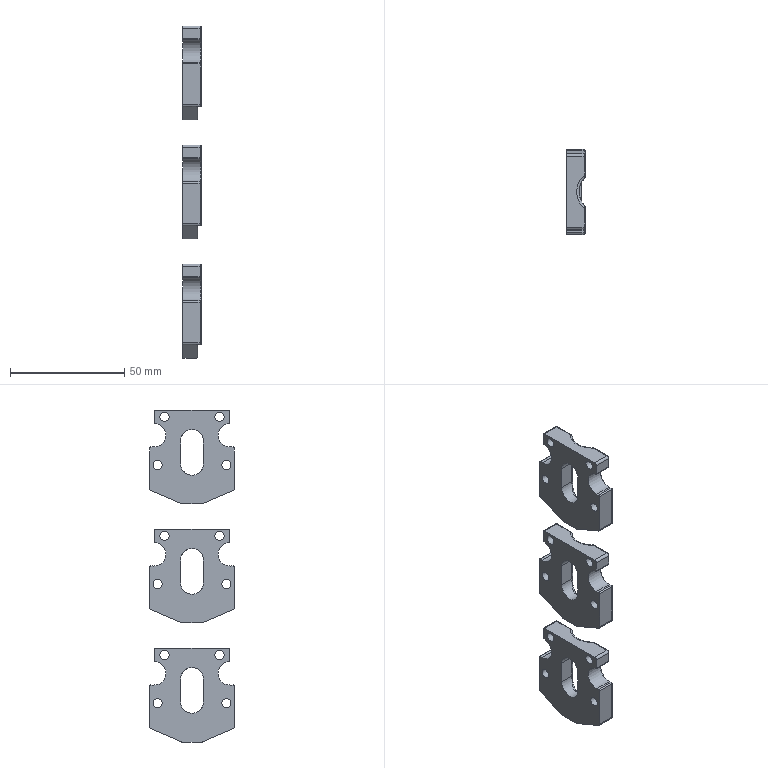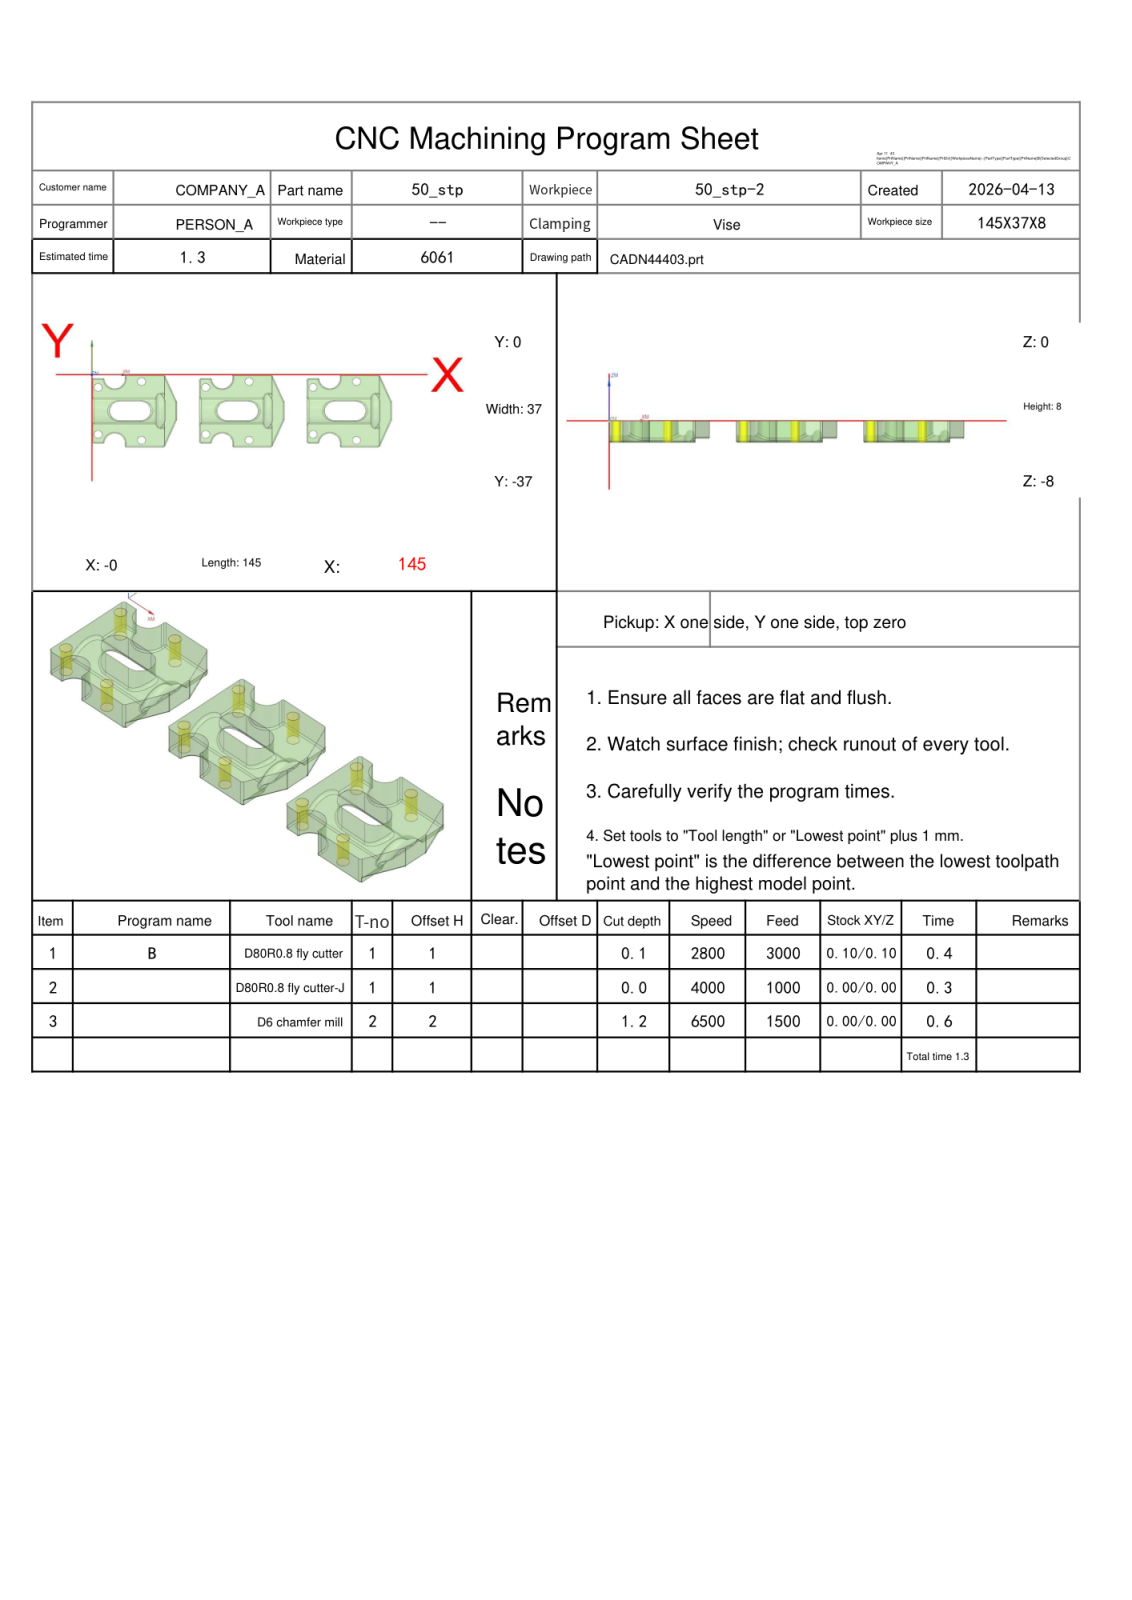NC program | NX | posted by the shop | part box 8 x 37 x 145 mm
Whole program:
%
O0001
(Machine time: 1.85 MIN)
(===Total Tool:2===)
(T1=D80R0.8 fly cutter D=80.  R=0.8  D-  H01 Z=-0.   )
(T2=D6 chamfer mill   D=6.   R=0.   D-  H02 Z=-1.2  )
G80 G90 G17 G49 G40
G91 G28 Z0
M01
N1 T01 M06
(D80R0.8 fly cutter  D=80. R=0.8 H=01 ce=0.10 di=0.10)
G00 G90 G54 X197.097 Y-18.5 M03 S2800
G43 H01 Z20.
M08
Z3.525
G01 Z1.525 F3000.
X185.097
X-40.097
X-52.097
Z3.525
G00 X197.097
Z3.05
G01 Z1.05
X185.097
X-40.097
X-52.097
Z3.05
G00 X197.097
Z2.575
G01 Z.575
X185.097
X-40.097
X-52.097
Z2.575
G00 X197.097
Z2.1
G01 Z.1
X185.097
X-40.097
X-52.097
Z2.1
G00 Z20.
G91 G28 Z0.0
M05
M09
G91 G28 Z0.0
M01
N2 T01 M06
(D80R0.8 fly cutter-J  D=80. R=0.8 H=01 ce=0.00 di=0.00)
G00 G90 G54 X196.999 Y-18.5 M03 S4000
G43 H01 Z20.
M08
Z2.
G01 Z0.0 F1000.
X184.999
X-39.999
X-51.999
Z2.
G00 Z20.
G91 G28 Z0.0
M05
M09
G91 G28 Z0.0
M01
N3 T02 M06
(D6 chamfer mill  D=6. R=0. H=02 ce=0.00 di=0.00)
G00 G90 G54 X102.773 Y-18.886 M03 S6500
G43 H02 Z20.
M08
Z.172
G01 Z-1.199 F1500.
G03 X102.973 Y-18.6 I-1.532 J1.286
G01 X103.003 Y-18.554
X103. Y-18.5
Y-3.
G02 X105. Y-1. I2. J0.0
G01 X109.372
G02 X110.866 Y-2.367 I0.0 J-1.5
G03 X115. Y-6.15 I4.134 J.367
X119.15 Y-2. I0.0 J4.15
X119.144 Y-1.777 I-4.15 J0.0
G01 X119.08 Y-.58
X119.078 Y-.5
G02 X120.578 Y1. I1.5 J0.0
G01 X138.341
G02 X140.179 Y-.212 I0.0 J-2.
G01 X145.879 Y-13.512
X145.969 Y-13.801
X146. Y-14.103
Y-22.897
X145.969 Y-23.199
X145.879 Y-23.488
X140.179 Y-36.788
G02 X138.341 Y-38. I-1.838 J.788
G01 X120.578
G02 X119.078 Y-36.5 I0.0 J1.5
G01 X119.08 Y-36.42
X119.144 Y-35.223
G03 X119.15 Y-35. I-4.144 J.223
X115. Y-30.85 I-4.15 J0.0
X110.866 Y-34.633 I0.0 J-4.15
G02 X109.372 Y-36. I-1.494 J.133
G01 X105.
G02 X103. Y-34. I0.0 J2.
G01 Y-18.5
X103.003 Y-18.446
X102.973 Y-18.4
G03 X102.773 Y-18.114 I-1.732 J-1.
G01 Z.172
G00 Z10.
X128.826 Y-33.912
Z.33
G01 Z-1.199
G03 X128.986 Y-33.603 I-1.687 J1.075
G01 X129.01 Y-33.554
X129. Y-33.5
G03 X128. Y-32.5 I-1. J0.0
X127. Y-33.5 I0.0 J-1.
X128. Y-34.5 I1. J0.0
X129. Y-33.5 I0.0 J1.
G01 X129.01 Y-33.446
X128.986 Y-33.397
G03 X128.826 Y-33.088 I-1.848 J-.765
G01 Z.33
G00 Z10.
X122.114 Y-22.273
Z.172
G01 Z-1.199
G03 X122.4 Y-22.473 I1.286 J1.532
G01 X122.446 Y-22.503
X122.5 Y-22.5
X127.5
G03 X131.5 Y-18.5 I0.0 J4.
X127.5 Y-14.5 I-4. J0.0
G01 X117.5
G03 X113.5 Y-18.5 I0.0 J-4.
X117.5 Y-22.5 I4. J0.0
G01 X122.5
X122.554 Y-22.503
X122.6 Y-22.473
G03 X122.886 Y-22.273 I-1. J1.732
G01 Z.172
G00 Z10.
X128.826 Y-3.912
Z.33
G01 Z-1.199
G03 X128.986 Y-3.603 I-1.687 J1.075
G01 X129.01 Y-3.554
X129. Y-3.5
G03 X128. Y-2.5 I-1. J0.0
X127. Y-3.5 I0.0 J-1.
X128. Y-4.5 I1. J0.0
X129. Y-3.5 I0.0 J1.
G01 X129.01 Y-3.446
X128.986 Y-3.397
G03 X128.826 Y-3.088 I-1.848 J-.765
G01 Z.33
G00 Z10.
X107.826 Y-6.912
Z.33
G01 Z-1.199
G03 X107.986 Y-6.603 I-1.687 J1.075
G01 X108.01 Y-6.554
X108. Y-6.5
G03 X107. Y-5.5 I-1. J0.0
X106. Y-6.5 I0.0 J-1.
X107. Y-7.5 I1. J0.0
X108. Y-6.5 I0.0 J1.
G01 X108.01 Y-6.446
X107.986 Y-6.397
G03 X107.826 Y-6.088 I-1.848 J-.765
G01 Z.33
G00 Z10.
Y-30.912
Z.33
G01 Z-1.199
G03 X107.986 Y-30.603 I-1.687 J1.075
G01 X108.01 Y-30.554
X108. Y-30.5
G03 X107. Y-29.5 I-1. J0.0
X106. Y-30.5 I0.0 J-1.
X107. Y-31.5 I1. J0.0
X108. Y-30.5 I0.0 J1.
G01 X108.01 Y-30.446
X107.986 Y-30.397
G03 X107.826 Y-30.088 I-1.848 J-.765
G01 Z.33
G00 Z10.
X50.773 Y-18.886
Z.172
G01 Z-1.199
G03 X50.973 Y-18.6 I-1.532 J1.286
G01 X51.003 Y-18.554
X51. Y-18.5
Y-3.
G02 X53. Y-1. I2. J0.0
G01 X57.372
G02 X58.866 Y-2.367 I0.0 J-1.5
G03 X63. Y-6.15 I4.134 J.367
X67.15 Y-2. I0.0 J4.15
X67.144 Y-1.777 I-4.15 J0.0
G01 X67.08 Y-.58
X67.078 Y-.5
G02 X68.578 Y1. I1.5 J0.0
G01 X86.341
G02 X88.179 Y-.212 I0.0 J-2.
G01 X93.879 Y-13.512
X93.969 Y-13.801
X94. Y-14.103
Y-22.897
X93.969 Y-23.199
X93.879 Y-23.488
X88.179 Y-36.788
G02 X86.341 Y-38. I-1.838 J.788
G01 X68.578
G02 X67.078 Y-36.5 I0.0 J1.5
G01 X67.08 Y-36.42
X67.144 Y-35.223
G03 X67.15 Y-35. I-4.144 J.223
X63. Y-30.85 I-4.15 J0.0
X58.866 Y-34.633 I0.0 J-4.15
G02 X57.372 Y-36. I-1.494 J.133
G01 X53.
G02 X51. Y-34. I0.0 J2.
G01 Y-18.5
X51.003 Y-18.446
X50.973 Y-18.4
G03 X50.773 Y-18.114 I-1.732 J-1.
G01 Z.172
G00 Z10.
X76.826 Y-33.912
Z.33
G01 Z-1.199
G03 X76.986 Y-33.603 I-1.687 J1.075
G01 X77.01 Y-33.554
X77. Y-33.5
G03 X76. Y-32.5 I-1. J0.0
X75. Y-33.5 I0.0 J-1.
X76. Y-34.5 I1. J0.0
X77. Y-33.5 I0.0 J1.
G01 X77.01 Y-33.446
X76.986 Y-33.397
G03 X76.826 Y-33.088 I-1.848 J-.765
G01 Z.33
G00 Z10.
X70.114 Y-22.273
Z.172
G01 Z-1.199
G03 X70.4 Y-22.473 I1.286 J1.532
G01 X70.446 Y-22.503
X70.5 Y-22.5
X75.5
G03 X79.5 Y-18.5 I0.0 J4.
X75.5 Y-14.5 I-4. J0.0
G01 X65.5
G03 X61.5 Y-18.5 I0.0 J-4.
X65.5 Y-22.5 I4. J0.0
G01 X70.5
X70.554 Y-22.503
X70.6 Y-22.473
G03 X70.886 Y-22.273 I-1. J1.732
G01 Z.172
G00 Z10.
X76.826 Y-3.912
Z.33
G01 Z-1.199
G03 X76.986 Y-3.603 I-1.687 J1.075
G01 X77.01 Y-3.554
X77. Y-3.5
G03 X76. Y-2.5 I-1. J0.0
X75. Y-3.5 I0.0 J-1.
X76. Y-4.5 I1. J0.0
X77. Y-3.5 I0.0 J1.
G01 X77.01 Y-3.446
X76.986 Y-3.397
G03 X76.826 Y-3.088 I-1.848 J-.765
G01 Z.33
G00 Z10.
X55.826 Y-6.912
Z.33
G01 Z-1.199
G03 X55.986 Y-6.603 I-1.687 J1.075
G01 X56.01 Y-6.554
X56. Y-6.5
G03 X55. Y-5.5 I-1. J0.0
X54. Y-6.5 I0.0 J-1.
X55. Y-7.5 I1. J0.0
X56. Y-6.5 I0.0 J1.
G01 X56.01 Y-6.446
X55.986 Y-6.397
G03 X55.826 Y-6.088 I-1.848 J-.765
G01 Z.33
G00 Z10.
Y-30.912
Z.33
G01 Z-1.199
G03 X55.986 Y-30.603 I-1.687 J1.075
G01 X56.01 Y-30.554
X56. Y-30.5
G03 X55. Y-29.5 I-1. J0.0
X54. Y-30.5 I0.0 J-1.
X55. Y-31.5 I1. J0.0
X56. Y-30.5 I0.0 J1.
G01 X56.01 Y-30.446
X55.986 Y-30.397
G03 X55.826 Y-30.088 I-1.848 J-.765
G01 Z.33
G00 Z10.
X-1.227 Y-18.886
Z.172
G01 Z-1.199
G03 X-1.027 Y-18.6 I-1.532 J1.286
G01 X-.997 Y-18.554
X-1. Y-18.5
Y-3.
G02 X1. Y-1. I2. J0.0
G01 X5.372
G02 X6.866 Y-2.367 I0.0 J-1.5
G03 X11. Y-6.15 I4.134 J.367
X15.15 Y-2. I0.0 J4.15
X15.144 Y-1.777 I-4.15 J0.0
G01 X15.08 Y-.58
X15.078 Y-.5
G02 X16.578 Y1. I1.5 J0.0
G01 X34.341
G02 X36.179 Y-.212 I0.0 J-2.
G01 X41.879 Y-13.512
X41.969 Y-13.801
X42. Y-14.103
Y-22.897
X41.969 Y-23.199
X41.879 Y-23.488
X36.179 Y-36.788
G02 X34.341 Y-38. I-1.838 J.788
G01 X16.578
G02 X15.078 Y-36.5 I0.0 J1.5
G01 X15.08 Y-36.42
X15.144 Y-35.223
G03 X15.15 Y-35. I-4.144 J.223
X11. Y-30.85 I-4.15 J0.0
X6.866 Y-34.633 I0.0 J-4.15
G02 X5.372 Y-36. I-1.494 J.133
G01 X1.
G02 X-1. Y-34. I0.0 J2.
G01 Y-18.5
X-.997 Y-18.446
X-1.027 Y-18.4
G03 X-1.227 Y-18.114 I-1.732 J-1.
G01 Z.172
G00 Z10.
X24.826 Y-33.912
Z.33
G01 Z-1.199
G03 X24.986 Y-33.603 I-1.687 J1.075
G01 X25.01 Y-33.554
X25. Y-33.5
G03 X24. Y-32.5 I-1. J0.0
X23. Y-33.5 I0.0 J-1.
X24. Y-34.5 I1. J0.0
X25. Y-33.5 I0.0 J1.
G01 X25.01 Y-33.446
X24.986 Y-33.397
G03 X24.826 Y-33.088 I-1.848 J-.765
G01 Z.33
G00 Z10.
X18.114 Y-22.273
Z.172
G01 Z-1.199
G03 X18.4 Y-22.473 I1.286 J1.532
G01 X18.446 Y-22.503
X18.5 Y-22.5
X23.5
G03 X27.5 Y-18.5 I0.0 J4.
X23.5 Y-14.5 I-4. J0.0
G01 X13.5
G03 X9.5 Y-18.5 I0.0 J-4.
X13.5 Y-22.5 I4. J0.0
G01 X18.5
X18.554 Y-22.503
X18.6 Y-22.473
G03 X18.886 Y-22.273 I-1. J1.732
G01 Z.172
G00 Z10.
X24.826 Y-3.912
Z.33
G01 Z-1.199
G03 X24.986 Y-3.603 I-1.687 J1.075
G01 X25.01 Y-3.554
X25. Y-3.5
G03 X24. Y-2.5 I-1. J0.0
X23. Y-3.5 I0.0 J-1.
X24. Y-4.5 I1. J0.0
X25. Y-3.5 I0.0 J1.
G01 X25.01 Y-3.446
X24.986 Y-3.397
G03 X24.826 Y-3.088 I-1.848 J-.765
G01 Z.33
G00 Z10.
X3.826 Y-6.912
Z.33
G01 Z-1.199
G03 X3.986 Y-6.603 I-1.687 J1.075
G01 X4.01 Y-6.554
X4. Y-6.5
G03 X3. Y-5.5 I-1. J0.0
X2. Y-6.5 I0.0 J-1.
X3. Y-7.5 I1. J0.0
X4. Y-6.5 I0.0 J1.
G01 X4.01 Y-6.446
X3.986 Y-6.397
G03 X3.826 Y-6.088 I-1.848 J-.765
G01 Z.33
G00 Z10.
Y-30.912
Z.33
G01 Z-1.199
G03 X3.986 Y-30.603 I-1.687 J1.075
G01 X4.01 Y-30.554
X4. Y-30.5
G03 X3. Y-29.5 I-1. J0.0
X2. Y-30.5 I0.0 J-1.
X3. Y-31.5 I1. J0.0
X4. Y-30.5 I0.0 J1.
G01 X4.01 Y-30.446
X3.986 Y-30.397
G03 X3.826 Y-30.088 I-1.848 J-.765
G01 Z.33
G00 Z20.
M05
M09
G91 G28 Z0.0
G91 G28 Y0.0
M30
%